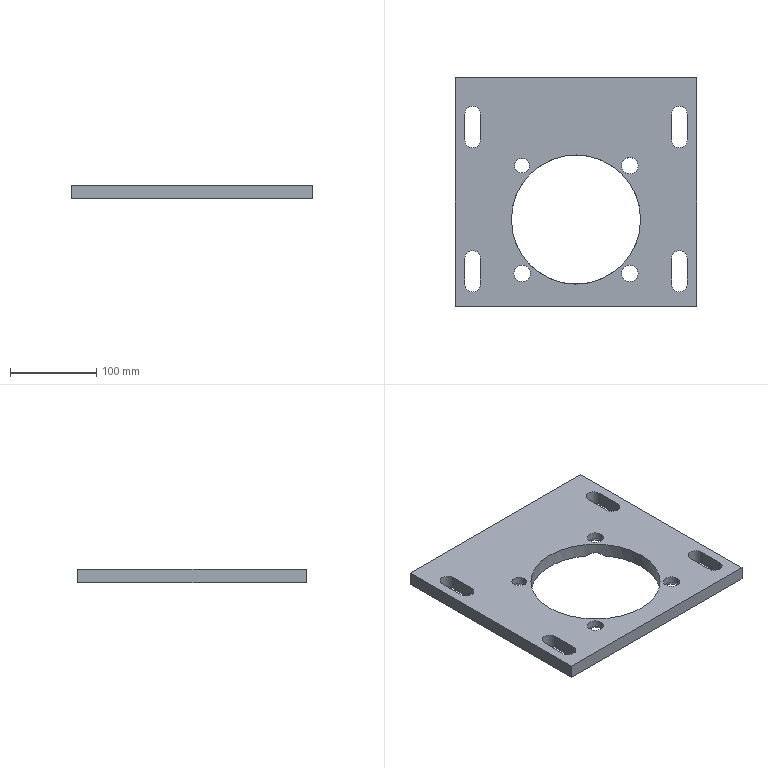Part | SolidWorks | features ICE 3, Extrusion 1 | 1 solid | 40 faces | box 280 x 265 x 16 mm | volume 827088 mm3 | cylinder 18 | plane 14 | cone 8 | commonest cylinder face diameters 18 x8 19 x6 17 x2 150 x2
STEP:
#1=CARTESIAN_POINT('',(-53.079,-62.579,0.));
#2=VERTEX_POINT('',#1);
#3=CARTESIAN_POINT('',(-72.079,-62.579,0.));
#4=VERTEX_POINT('',#3);
#5=CARTESIAN_POINT('',(-62.579,-62.579,0.));
#6=DIRECTION('',(0.,0.,1.));
#7=DIRECTION('',(1.,0.,0.));
#8=AXIS2_PLACEMENT_3D('',#5,#6,#7);
#9=CIRCLE('',#8,9.5);
#10=EDGE_CURVE('',#2,#4,#9,.T.);
#11=ORIENTED_EDGE('',*,*,#10,.T.);
#12=CARTESIAN_POINT('',(-80.079,-62.579,-8.));
#13=VERTEX_POINT('',#12);
#14=CARTESIAN_POINT('',(-72.079,-62.579,0.));
#15=DIRECTION('',(-0.7071,0.,-0.7071));
#16=VECTOR('',#15,1000.);
#17=LINE('',#14,#16);
#18=EDGE_CURVE('',#4,#13,#17,.T.);
#19=ORIENTED_EDGE('',*,*,#18,.T.);
#20=CARTESIAN_POINT('',(-59.769,-45.306,-8.));
#21=VERTEX_POINT('',#20);
#22=CARTESIAN_POINT('',(-62.579,-62.579,-8.));
#23=DIRECTION('',(0.,0.,1.));
#24=DIRECTION('',(1.,0.,0.));
#25=AXIS2_PLACEMENT_3D('',#22,#23,#24);
#26=CIRCLE('',#25,17.5);
#27=EDGE_CURVE('',#21,#13,#26,.T.);
#28=ORIENTED_EDGE('',*,*,#27,.F.);
#29=CARTESIAN_POINT('',(-45.306,-59.769,-8.));
#30=VERTEX_POINT('',#29);
#31=CARTESIAN_POINT('',(-59.769,-45.306,-8.));
#32=CARTESIAN_POINT('',(-59.304,-45.92,-7.469));
#33=CARTESIAN_POINT('',(-58.822,-46.537,-6.963));
#34=CARTESIAN_POINT('',(-57.811,-47.787,-6.028));
#35=CARTESIAN_POINT('',(-57.282,-48.42,-5.598));
#36=CARTESIAN_POINT('',(-56.442,-49.391,-5.041));
#37=CARTESIAN_POINT('',(-56.153,-49.72,-4.869));
#38=CARTESIAN_POINT('',(-55.56,-50.381,-4.567));
#39=CARTESIAN_POINT('',(-55.258,-50.712,-4.436));
#40=CARTESIAN_POINT('',(-54.642,-51.376,-4.223));
#41=CARTESIAN_POINT('',(-54.327,-51.708,-4.14));
#42=CARTESIAN_POINT('',(-53.685,-52.375,-4.028));
#43=CARTESIAN_POINT('',(-53.355,-52.711,-3.999));
#44=CARTESIAN_POINT('',(-52.358,-53.707,-4.001));
#45=CARTESIAN_POINT('',(-51.694,-54.346,-4.119));
#46=CARTESIAN_POINT('',(-50.697,-55.272,-4.442));
#47=CARTESIAN_POINT('',(-50.363,-55.576,-4.574));
#48=CARTESIAN_POINT('',(-49.702,-56.168,-4.878));
#49=CARTESIAN_POINT('',(-49.377,-56.455,-5.049));
#50=CARTESIAN_POINT('',(-48.41,-57.29,-5.604));
#51=CARTESIAN_POINT('',(-47.78,-57.816,-6.033));
#52=CARTESIAN_POINT('',(-46.534,-58.824,-6.966));
#53=CARTESIAN_POINT('',(-45.918,-59.305,-7.47));
#54=CARTESIAN_POINT('',(-45.306,-59.769,-8.));
#55=B_SPLINE_CURVE_WITH_KNOTS('',3,(#31,#32,#33,#34,#35,#36,#37,#38,#39,#40,#41,#42,#43,#44,#45,#46,#47,#48,#49,#50,#51,#52,#53,#54),.UNSPECIFIED.,.F.,.F.,(4,2,2,2,2,2,2,2,2,2,2,4),(0.00000035,0.002789,0.005578,0.006972,0.008366,0.009761,0.01116,0.01394,0.01534,0.01673,0.01952,0.02231),.UNSPECIFIED.);
#56=EDGE_CURVE('',#21,#30,#55,.T.);
#57=ORIENTED_EDGE('',*,*,#56,.T.);
#58=CARTESIAN_POINT('',(-45.079,-62.579,-8.));
#59=VERTEX_POINT('',#58);
#60=CARTESIAN_POINT('',(-62.579,-62.579,-8.));
#61=DIRECTION('',(0.,0.,1.));
#62=DIRECTION('',(1.,0.,0.));
#63=AXIS2_PLACEMENT_3D('',#60,#61,#62);
#64=CIRCLE('',#63,17.5);
#65=EDGE_CURVE('',#59,#30,#64,.T.);
#66=ORIENTED_EDGE('',*,*,#65,.F.);
#67=CARTESIAN_POINT('',(-53.079,-62.579,0.));
#68=DIRECTION('',(0.7071,0.,-0.7071));
#69=VECTOR('',#68,1000.);
#70=LINE('',#67,#69);
#71=EDGE_CURVE('',#2,#59,#70,.T.);
#72=ORIENTED_EDGE('',*,*,#71,.F.);
#73=EDGE_LOOP('',(#11,#19,#28,#57,#66,#72));
#74=FACE_OUTER_BOUND('',#73,.T.);
#75=CARTESIAN_POINT('',(-62.579,-62.579,0.));
#76=DIRECTION('',(0.,0.,-1.));
#77=DIRECTION('',(1.,0.,0.));
#78=AXIS2_PLACEMENT_3D('',#75,#76,#77);
#79=CONICAL_SURFACE('',#78,9.5,0.7854);
#80=ADVANCED_FACE('',(#74),#79,.F.);
#81=CARTESIAN_POINT('',(72.079,-62.579,0.));
#82=VERTEX_POINT('',#81);
#83=CARTESIAN_POINT('',(53.079,-62.579,0.));
#84=VERTEX_POINT('',#83);
#85=CARTESIAN_POINT('',(62.579,-62.579,0.));
#86=DIRECTION('',(0.,0.,1.));
#87=DIRECTION('',(1.,0.,0.));
#88=AXIS2_PLACEMENT_3D('',#85,#86,#87);
#89=CIRCLE('',#88,9.5);
#90=EDGE_CURVE('',#82,#84,#89,.T.);
#91=ORIENTED_EDGE('',*,*,#90,.T.);
#92=CARTESIAN_POINT('',(45.079,-62.579,-8.));
#93=VERTEX_POINT('',#92);
#94=CARTESIAN_POINT('',(53.079,-62.579,0.));
#95=DIRECTION('',(-0.7071,0.,-0.7071));
#96=VECTOR('',#95,1000.);
#97=LINE('',#94,#96);
#98=EDGE_CURVE('',#84,#93,#97,.T.);
#99=ORIENTED_EDGE('',*,*,#98,.T.);
#100=CARTESIAN_POINT('',(45.306,-59.769,-8.));
#101=VERTEX_POINT('',#100);
#102=CARTESIAN_POINT('',(62.579,-62.579,-8.));
#103=DIRECTION('',(0.,0.,1.));
#104=DIRECTION('',(1.,0.,0.));
#105=AXIS2_PLACEMENT_3D('',#102,#103,#104);
#106=CIRCLE('',#105,17.5);
#107=EDGE_CURVE('',#101,#93,#106,.T.);
#108=ORIENTED_EDGE('',*,*,#107,.F.);
#109=CARTESIAN_POINT('',(59.769,-45.306,-8.));
#110=VERTEX_POINT('',#109);
#111=CARTESIAN_POINT('',(45.306,-59.769,-8.));
#112=CARTESIAN_POINT('',(45.92,-59.304,-7.469));
#113=CARTESIAN_POINT('',(46.537,-58.822,-6.963));
#114=CARTESIAN_POINT('',(47.787,-57.811,-6.028));
#115=CARTESIAN_POINT('',(48.42,-57.282,-5.598));
#116=CARTESIAN_POINT('',(49.391,-56.442,-5.041));
#117=CARTESIAN_POINT('',(49.72,-56.153,-4.869));
#118=CARTESIAN_POINT('',(50.381,-55.56,-4.567));
#119=CARTESIAN_POINT('',(50.712,-55.258,-4.436));
#120=CARTESIAN_POINT('',(51.376,-54.642,-4.223));
#121=CARTESIAN_POINT('',(51.708,-54.327,-4.14));
#122=CARTESIAN_POINT('',(52.375,-53.685,-4.028));
#123=CARTESIAN_POINT('',(52.711,-53.355,-3.999));
#124=CARTESIAN_POINT('',(53.707,-52.358,-4.001));
#125=CARTESIAN_POINT('',(54.346,-51.694,-4.119));
#126=CARTESIAN_POINT('',(55.272,-50.697,-4.442));
#127=CARTESIAN_POINT('',(55.576,-50.363,-4.574));
#128=CARTESIAN_POINT('',(56.168,-49.702,-4.878));
#129=CARTESIAN_POINT('',(56.455,-49.377,-5.049));
#130=CARTESIAN_POINT('',(57.29,-48.41,-5.604));
#131=CARTESIAN_POINT('',(57.816,-47.78,-6.033));
#132=CARTESIAN_POINT('',(58.824,-46.534,-6.966));
#133=CARTESIAN_POINT('',(59.305,-45.918,-7.47));
#134=CARTESIAN_POINT('',(59.769,-45.306,-8.));
#135=B_SPLINE_CURVE_WITH_KNOTS('',3,(#111,#112,#113,#114,#115,#116,#117,#118,#119,#120,#121,#122,#123,#124,#125,#126,#127,#128,#129,#130,#131,#132,#133,#134),.UNSPECIFIED.,.F.,.F.,(4,2,2,2,2,2,2,2,2,2,2,4),(0.00000035,0.002789,0.005578,0.006972,0.008366,0.009761,0.01116,0.01394,0.01534,0.01673,0.01952,0.02231),.UNSPECIFIED.);
#136=EDGE_CURVE('',#101,#110,#135,.T.);
#137=ORIENTED_EDGE('',*,*,#136,.T.);
#138=CARTESIAN_POINT('',(80.079,-62.579,-8.));
#139=VERTEX_POINT('',#138);
#140=CARTESIAN_POINT('',(62.579,-62.579,-8.));
#141=DIRECTION('',(0.,0.,1.));
#142=DIRECTION('',(1.,0.,0.));
#143=AXIS2_PLACEMENT_3D('',#140,#141,#142);
#144=CIRCLE('',#143,17.5);
#145=EDGE_CURVE('',#139,#110,#144,.T.);
#146=ORIENTED_EDGE('',*,*,#145,.F.);
#147=CARTESIAN_POINT('',(72.079,-62.579,0.));
#148=DIRECTION('',(0.7071,0.,-0.7071));
#149=VECTOR('',#148,1000.);
#150=LINE('',#147,#149);
#151=EDGE_CURVE('',#82,#139,#150,.T.);
#152=ORIENTED_EDGE('',*,*,#151,.F.);
#153=EDGE_LOOP('',(#91,#99,#108,#137,#146,#152));
#154=FACE_OUTER_BOUND('',#153,.T.);
#155=CARTESIAN_POINT('',(62.579,-62.579,0.));
#156=DIRECTION('',(0.,0.,-1.));
#157=DIRECTION('',(1.,0.,0.));
#158=AXIS2_PLACEMENT_3D('',#155,#156,#157);
#159=CONICAL_SURFACE('',#158,9.5,0.7854);
#160=ADVANCED_FACE('',(#154),#159,.F.);
#161=CARTESIAN_POINT('',(72.079,62.579,0.));
#162=VERTEX_POINT('',#161);
#163=CARTESIAN_POINT('',(53.079,62.579,0.));
#164=VERTEX_POINT('',#163);
#165=CARTESIAN_POINT('',(62.579,62.579,0.));
#166=DIRECTION('',(0.,0.,1.));
#167=DIRECTION('',(1.,0.,0.));
#168=AXIS2_PLACEMENT_3D('',#165,#166,#167);
#169=CIRCLE('',#168,9.5);
#170=EDGE_CURVE('',#162,#164,#169,.T.);
#171=ORIENTED_EDGE('',*,*,#170,.T.);
#172=CARTESIAN_POINT('',(45.079,62.579,-8.));
#173=VERTEX_POINT('',#172);
#174=CARTESIAN_POINT('',(53.079,62.579,0.));
#175=DIRECTION('',(-0.7071,0.,-0.7071));
#176=VECTOR('',#175,1000.);
#177=LINE('',#174,#176);
#178=EDGE_CURVE('',#164,#173,#177,.T.);
#179=ORIENTED_EDGE('',*,*,#178,.T.);
#180=CARTESIAN_POINT('',(80.079,62.579,-8.));
#181=VERTEX_POINT('',#180);
#182=CARTESIAN_POINT('',(62.579,62.579,-8.));
#183=DIRECTION('',(0.,0.,1.));
#184=DIRECTION('',(1.,0.,0.));
#185=AXIS2_PLACEMENT_3D('',#182,#183,#184);
#186=CIRCLE('',#185,17.5);
#187=EDGE_CURVE('',#181,#173,#186,.T.);
#188=ORIENTED_EDGE('',*,*,#187,.F.);
#189=CARTESIAN_POINT('',(72.079,62.579,0.));
#190=DIRECTION('',(0.7071,0.,-0.7071));
#191=VECTOR('',#190,1000.);
#192=LINE('',#189,#191);
#193=EDGE_CURVE('',#162,#181,#192,.T.);
#194=ORIENTED_EDGE('',*,*,#193,.F.);
#195=EDGE_LOOP('',(#171,#179,#188,#194));
#196=FACE_OUTER_BOUND('',#195,.T.);
#197=CARTESIAN_POINT('',(62.579,62.579,0.));
#198=DIRECTION('',(0.,0.,-1.));
#199=DIRECTION('',(1.,0.,0.));
#200=AXIS2_PLACEMENT_3D('',#197,#198,#199);
#201=CONICAL_SURFACE('',#200,9.5,0.7854);
#202=ADVANCED_FACE('',(#196),#201,.F.);
#203=CARTESIAN_POINT('',(-54.079,62.579,0.));
#204=VERTEX_POINT('',#203);
#205=CARTESIAN_POINT('',(-71.079,62.579,0.));
#206=VERTEX_POINT('',#205);
#207=CARTESIAN_POINT('',(-62.579,62.579,0.));
#208=DIRECTION('',(0.,0.,1.));
#209=DIRECTION('',(1.,0.,0.));
#210=AXIS2_PLACEMENT_3D('',#207,#208,#209);
#211=CIRCLE('',#210,8.5);
#212=EDGE_CURVE('',#204,#206,#211,.T.);
#213=ORIENTED_EDGE('',*,*,#212,.T.);
#214=CARTESIAN_POINT('',(-79.079,62.579,-8.));
#215=VERTEX_POINT('',#214);
#216=CARTESIAN_POINT('',(-71.079,62.579,0.));
#217=DIRECTION('',(-0.7071,0.,-0.7071));
#218=VECTOR('',#217,1000.);
#219=LINE('',#216,#218);
#220=EDGE_CURVE('',#206,#215,#219,.T.);
#221=ORIENTED_EDGE('',*,*,#220,.T.);
#222=CARTESIAN_POINT('',(-46.079,62.579,-8.));
#223=VERTEX_POINT('',#222);
#224=CARTESIAN_POINT('',(-62.579,62.579,-8.));
#225=DIRECTION('',(0.,0.,1.));
#226=DIRECTION('',(1.,0.,0.));
#227=AXIS2_PLACEMENT_3D('',#224,#225,#226);
#228=CIRCLE('',#227,16.5);
#229=EDGE_CURVE('',#223,#215,#228,.T.);
#230=ORIENTED_EDGE('',*,*,#229,.F.);
#231=CARTESIAN_POINT('',(-54.079,62.579,0.));
#232=DIRECTION('',(0.7071,0.,-0.7071));
#233=VECTOR('',#232,1000.);
#234=LINE('',#231,#233);
#235=EDGE_CURVE('',#204,#223,#234,.T.);
#236=ORIENTED_EDGE('',*,*,#235,.F.);
#237=EDGE_LOOP('',(#213,#221,#230,#236));
#238=FACE_OUTER_BOUND('',#237,.T.);
#239=CARTESIAN_POINT('',(-62.579,62.579,0.));
#240=DIRECTION('',(0.,0.,-1.));
#241=DIRECTION('',(1.,0.,0.));
#242=AXIS2_PLACEMENT_3D('',#239,#240,#241);
#243=CONICAL_SURFACE('',#242,8.5,0.7854);
#244=ADVANCED_FACE('',(#238),#243,.F.);
#245=CARTESIAN_POINT('',(-62.579,-62.579,0.));
#246=DIRECTION('',(0.,0.,1.));
#247=DIRECTION('',(1.,0.,0.));
#248=AXIS2_PLACEMENT_3D('',#245,#246,#247);
#249=CIRCLE('',#248,9.5);
#250=EDGE_CURVE('',#4,#2,#249,.T.);
#251=ORIENTED_EDGE('',*,*,#250,.F.);
#252=CARTESIAN_POINT('',(-72.079,-62.579,8.));
#253=VERTEX_POINT('',#252);
#254=CARTESIAN_POINT('',(-72.079,-62.579,0.));
#255=DIRECTION('',(0.,0.,1.));
#256=VECTOR('',#255,1000.);
#257=LINE('',#254,#256);
#258=EDGE_CURVE('',#4,#253,#257,.T.);
#259=ORIENTED_EDGE('',*,*,#258,.T.);
#260=CARTESIAN_POINT('',(-53.079,-62.579,8.));
#261=VERTEX_POINT('',#260);
#262=CARTESIAN_POINT('',(-62.579,-62.579,8.));
#263=DIRECTION('',(0.,0.,1.));
#264=DIRECTION('',(1.,0.,0.));
#265=AXIS2_PLACEMENT_3D('',#262,#263,#264);
#266=CIRCLE('',#265,9.5);
#267=EDGE_CURVE('',#253,#261,#266,.T.);
#268=ORIENTED_EDGE('',*,*,#267,.T.);
#269=CARTESIAN_POINT('',(-53.079,-62.579,0.));
#270=DIRECTION('',(0.,0.,1.));
#271=VECTOR('',#270,1000.);
#272=LINE('',#269,#271);
#273=EDGE_CURVE('',#2,#261,#272,.T.);
#274=ORIENTED_EDGE('',*,*,#273,.F.);
#275=EDGE_LOOP('',(#251,#259,#268,#274));
#276=FACE_OUTER_BOUND('',#275,.T.);
#277=CARTESIAN_POINT('',(-62.579,-62.579,0.));
#278=DIRECTION('',(0.,0.,1.));
#279=DIRECTION('',(1.,0.,0.));
#280=AXIS2_PLACEMENT_3D('',#277,#278,#279);
#281=CYLINDRICAL_SURFACE('',#280,9.5);
#282=ADVANCED_FACE('',(#276),#281,.F.);
#283=CARTESIAN_POINT('',(62.579,-62.579,0.));
#284=DIRECTION('',(0.,0.,1.));
#285=DIRECTION('',(1.,0.,0.));
#286=AXIS2_PLACEMENT_3D('',#283,#284,#285);
#287=CIRCLE('',#286,9.5);
#288=EDGE_CURVE('',#84,#82,#287,.T.);
#289=ORIENTED_EDGE('',*,*,#288,.F.);
#290=CARTESIAN_POINT('',(53.079,-62.579,8.));
#291=VERTEX_POINT('',#290);
#292=CARTESIAN_POINT('',(53.079,-62.579,0.));
#293=DIRECTION('',(0.,0.,1.));
#294=VECTOR('',#293,1000.);
#295=LINE('',#292,#294);
#296=EDGE_CURVE('',#84,#291,#295,.T.);
#297=ORIENTED_EDGE('',*,*,#296,.T.);
#298=CARTESIAN_POINT('',(72.079,-62.579,8.));
#299=VERTEX_POINT('',#298);
#300=CARTESIAN_POINT('',(62.579,-62.579,8.));
#301=DIRECTION('',(0.,0.,1.));
#302=DIRECTION('',(1.,0.,0.));
#303=AXIS2_PLACEMENT_3D('',#300,#301,#302);
#304=CIRCLE('',#303,9.5);
#305=EDGE_CURVE('',#291,#299,#304,.T.);
#306=ORIENTED_EDGE('',*,*,#305,.T.);
#307=CARTESIAN_POINT('',(72.079,-62.579,0.));
#308=DIRECTION('',(0.,0.,1.));
#309=VECTOR('',#308,1000.);
#310=LINE('',#307,#309);
#311=EDGE_CURVE('',#82,#299,#310,.T.);
#312=ORIENTED_EDGE('',*,*,#311,.F.);
#313=EDGE_LOOP('',(#289,#297,#306,#312));
#314=FACE_OUTER_BOUND('',#313,.T.);
#315=CARTESIAN_POINT('',(62.579,-62.579,0.));
#316=DIRECTION('',(0.,0.,1.));
#317=DIRECTION('',(1.,0.,0.));
#318=AXIS2_PLACEMENT_3D('',#315,#316,#317);
#319=CYLINDRICAL_SURFACE('',#318,9.5);
#320=ADVANCED_FACE('',(#314),#319,.F.);
#321=CARTESIAN_POINT('',(62.579,62.579,0.));
#322=DIRECTION('',(0.,0.,1.));
#323=DIRECTION('',(1.,0.,0.));
#324=AXIS2_PLACEMENT_3D('',#321,#322,#323);
#325=CIRCLE('',#324,9.5);
#326=EDGE_CURVE('',#164,#162,#325,.T.);
#327=ORIENTED_EDGE('',*,*,#326,.F.);
#328=CARTESIAN_POINT('',(53.079,62.579,8.));
#329=VERTEX_POINT('',#328);
#330=CARTESIAN_POINT('',(53.079,62.579,0.));
#331=DIRECTION('',(0.,0.,1.));
#332=VECTOR('',#331,1000.);
#333=LINE('',#330,#332);
#334=EDGE_CURVE('',#164,#329,#333,.T.);
#335=ORIENTED_EDGE('',*,*,#334,.T.);
#336=CARTESIAN_POINT('',(72.079,62.579,8.));
#337=VERTEX_POINT('',#336);
#338=CARTESIAN_POINT('',(62.579,62.579,8.));
#339=DIRECTION('',(0.,0.,1.));
#340=DIRECTION('',(1.,0.,0.));
#341=AXIS2_PLACEMENT_3D('',#338,#339,#340);
#342=CIRCLE('',#341,9.5);
#343=EDGE_CURVE('',#329,#337,#342,.T.);
#344=ORIENTED_EDGE('',*,*,#343,.T.);
#345=CARTESIAN_POINT('',(72.079,62.579,0.));
#346=DIRECTION('',(0.,0.,1.));
#347=VECTOR('',#346,1000.);
#348=LINE('',#345,#347);
#349=EDGE_CURVE('',#162,#337,#348,.T.);
#350=ORIENTED_EDGE('',*,*,#349,.F.);
#351=EDGE_LOOP('',(#327,#335,#344,#350));
#352=FACE_OUTER_BOUND('',#351,.T.);
#353=CARTESIAN_POINT('',(62.579,62.579,0.));
#354=DIRECTION('',(0.,0.,1.));
#355=DIRECTION('',(1.,0.,0.));
#356=AXIS2_PLACEMENT_3D('',#353,#354,#355);
#357=CYLINDRICAL_SURFACE('',#356,9.5);
#358=ADVANCED_FACE('',(#352),#357,.F.);
#359=CARTESIAN_POINT('',(-62.579,62.579,0.));
#360=DIRECTION('',(0.,0.,1.));
#361=DIRECTION('',(1.,0.,0.));
#362=AXIS2_PLACEMENT_3D('',#359,#360,#361);
#363=CIRCLE('',#362,8.5);
#364=EDGE_CURVE('',#206,#204,#363,.T.);
#365=ORIENTED_EDGE('',*,*,#364,.F.);
#366=CARTESIAN_POINT('',(-71.079,62.579,8.));
#367=VERTEX_POINT('',#366);
#368=CARTESIAN_POINT('',(-71.079,62.579,0.));
#369=DIRECTION('',(0.,0.,1.));
#370=VECTOR('',#369,1000.);
#371=LINE('',#368,#370);
#372=EDGE_CURVE('',#206,#367,#371,.T.);
#373=ORIENTED_EDGE('',*,*,#372,.T.);
#374=CARTESIAN_POINT('',(-54.079,62.579,8.));
#375=VERTEX_POINT('',#374);
#376=CARTESIAN_POINT('',(-62.579,62.579,8.));
#377=DIRECTION('',(0.,0.,1.));
#378=DIRECTION('',(1.,0.,0.));
#379=AXIS2_PLACEMENT_3D('',#376,#377,#378);
#380=CIRCLE('',#379,8.5);
#381=EDGE_CURVE('',#367,#375,#380,.T.);
#382=ORIENTED_EDGE('',*,*,#381,.T.);
#383=CARTESIAN_POINT('',(-54.079,62.579,0.));
#384=DIRECTION('',(0.,0.,1.));
#385=VECTOR('',#384,1000.);
#386=LINE('',#383,#385);
#387=EDGE_CURVE('',#204,#375,#386,.T.);
#388=ORIENTED_EDGE('',*,*,#387,.F.);
#389=EDGE_LOOP('',(#365,#373,#382,#388));
#390=FACE_OUTER_BOUND('',#389,.T.);
#391=CARTESIAN_POINT('',(-62.579,62.579,0.));
#392=DIRECTION('',(0.,0.,1.));
#393=DIRECTION('',(1.,0.,0.));
#394=AXIS2_PLACEMENT_3D('',#391,#392,#393);
#395=CYLINDRICAL_SURFACE('',#394,8.5);
#396=ADVANCED_FACE('',(#390),#395,.F.);
#397=CARTESIAN_POINT('',(-75.,0.,8.));
#398=VERTEX_POINT('',#397);
#399=CARTESIAN_POINT('',(75.,0.,8.));
#400=VERTEX_POINT('',#399);
#401=CARTESIAN_POINT('',(0.,0.,8.));
#402=DIRECTION('',(0.,0.,1.));
#403=DIRECTION('',(1.,0.,0.));
#404=AXIS2_PLACEMENT_3D('',#401,#402,#403);
#405=CIRCLE('',#404,75.);
#406=EDGE_CURVE('',#398,#400,#405,.T.);
#407=ORIENTED_EDGE('',*,*,#406,.T.);
#408=CARTESIAN_POINT('',(75.,0.,-8.));
#409=VERTEX_POINT('',#408);
#410=CARTESIAN_POINT('',(75.,0.,8.));
#411=DIRECTION('',(0.,0.,-1.));
#412=VECTOR('',#411,1000.);
#413=LINE('',#410,#412);
#414=EDGE_CURVE('',#400,#409,#413,.T.);
#415=ORIENTED_EDGE('',*,*,#414,.T.);
#416=CARTESIAN_POINT('',(0.,0.,-8.));
#417=DIRECTION('',(0.,0.,1.));
#418=DIRECTION('',(1.,0.,0.));
#419=AXIS2_PLACEMENT_3D('',#416,#417,#418);
#420=CIRCLE('',#419,75.);
#421=EDGE_CURVE('',#110,#409,#420,.T.);
#422=ORIENTED_EDGE('',*,*,#421,.F.);
#423=ORIENTED_EDGE('',*,*,#136,.F.);
#424=CARTESIAN_POINT('',(0.,0.,-8.));
#425=DIRECTION('',(0.,0.,1.));
#426=DIRECTION('',(1.,0.,0.));
#427=AXIS2_PLACEMENT_3D('',#424,#425,#426);
#428=CIRCLE('',#427,75.);
#429=EDGE_CURVE('',#30,#101,#428,.T.);
#430=ORIENTED_EDGE('',*,*,#429,.F.);
#431=ORIENTED_EDGE('',*,*,#56,.F.);
#432=CARTESIAN_POINT('',(-75.,0.,-8.));
#433=VERTEX_POINT('',#432);
#434=CARTESIAN_POINT('',(0.,0.,-8.));
#435=DIRECTION('',(0.,0.,1.));
#436=DIRECTION('',(1.,0.,0.));
#437=AXIS2_PLACEMENT_3D('',#434,#435,#436);
#438=CIRCLE('',#437,75.);
#439=EDGE_CURVE('',#433,#21,#438,.T.);
#440=ORIENTED_EDGE('',*,*,#439,.F.);
#441=CARTESIAN_POINT('',(-75.,0.,8.));
#442=DIRECTION('',(0.,0.,-1.));
#443=VECTOR('',#442,1000.);
#444=LINE('',#441,#443);
#445=EDGE_CURVE('',#398,#433,#444,.T.);
#446=ORIENTED_EDGE('',*,*,#445,.F.);
#447=EDGE_LOOP('',(#407,#415,#422,#423,#430,#431,#440,#446));
#448=FACE_OUTER_BOUND('',#447,.T.);
#449=CARTESIAN_POINT('',(0.,0.,8.));
#450=DIRECTION('',(0.,0.,-1.));
#451=DIRECTION('',(-1.,0.,0.));
#452=AXIS2_PLACEMENT_3D('',#449,#450,#451);
#453=CYLINDRICAL_SURFACE('',#452,75.);
#454=ADVANCED_FACE('',(#448),#453,.F.);
#455=CARTESIAN_POINT('',(140.,-100.5,8.));
#456=VERTEX_POINT('',#455);
#457=CARTESIAN_POINT('',(-140.,-100.5,8.));
#458=VERTEX_POINT('',#457);
#459=CARTESIAN_POINT('',(-140.,-100.5,8.));
#460=DIRECTION('',(-1.,0.,0.));
#461=VECTOR('',#460,1000.);
#462=LINE('',#459,#461);
#463=EDGE_CURVE('',#456,#458,#462,.T.);
#464=ORIENTED_EDGE('',*,*,#463,.F.);
#465=CARTESIAN_POINT('',(140.,164.5,8.));
#466=VERTEX_POINT('',#465);
#467=CARTESIAN_POINT('',(140.,-115.5,8.));
#468=DIRECTION('',(0.,1.,0.));
#469=VECTOR('',#468,1000.);
#470=LINE('',#467,#469);
#471=EDGE_CURVE('',#456,#466,#470,.T.);
#472=ORIENTED_EDGE('',*,*,#471,.T.);
#473=CARTESIAN_POINT('',(-140.,164.5,8.));
#474=VERTEX_POINT('',#473);
#475=CARTESIAN_POINT('',(140.,164.5,8.));
#476=DIRECTION('',(-1.,0.,0.));
#477=VECTOR('',#476,1000.);
#478=LINE('',#475,#477);
#479=EDGE_CURVE('',#466,#474,#478,.T.);
#480=ORIENTED_EDGE('',*,*,#479,.T.);
#481=CARTESIAN_POINT('',(-140.,164.5,8.));
#482=DIRECTION('',(0.,-1.,0.));
#483=VECTOR('',#482,1000.);
#484=LINE('',#481,#483);
#485=EDGE_CURVE('',#474,#458,#484,.T.);
#486=ORIENTED_EDGE('',*,*,#485,.T.);
#487=EDGE_LOOP('',(#464,#472,#480,#486));
#488=FACE_OUTER_BOUND('',#487,.T.);
#489=CARTESIAN_POINT('',(-62.579,-62.579,8.));
#490=DIRECTION('',(0.,0.,1.));
#491=DIRECTION('',(1.,0.,0.));
#492=AXIS2_PLACEMENT_3D('',#489,#490,#491);
#493=CIRCLE('',#492,9.5);
#494=EDGE_CURVE('',#261,#253,#493,.T.);
#495=ORIENTED_EDGE('',*,*,#494,.F.);
#496=ORIENTED_EDGE('',*,*,#267,.F.);
#497=EDGE_LOOP('',(#495,#496));
#498=FACE_BOUND('',#497,.T.);
#499=CARTESIAN_POINT('',(62.579,-62.579,8.));
#500=DIRECTION('',(0.,0.,1.));
#501=DIRECTION('',(1.,0.,0.));
#502=AXIS2_PLACEMENT_3D('',#499,#500,#501);
#503=CIRCLE('',#502,9.5);
#504=EDGE_CURVE('',#299,#291,#503,.T.);
#505=ORIENTED_EDGE('',*,*,#504,.F.);
#506=ORIENTED_EDGE('',*,*,#305,.F.);
#507=EDGE_LOOP('',(#505,#506));
#508=FACE_BOUND('',#507,.T.);
#509=CARTESIAN_POINT('',(62.579,62.579,8.));
#510=DIRECTION('',(0.,0.,1.));
#511=DIRECTION('',(1.,0.,0.));
#512=AXIS2_PLACEMENT_3D('',#509,#510,#511);
#513=CIRCLE('',#512,9.5);
#514=EDGE_CURVE('',#337,#329,#513,.T.);
#515=ORIENTED_EDGE('',*,*,#514,.F.);
#516=ORIENTED_EDGE('',*,*,#343,.F.);
#517=EDGE_LOOP('',(#515,#516));
#518=FACE_BOUND('',#517,.T.);
#519=CARTESIAN_POINT('',(-62.579,62.579,8.));
#520=DIRECTION('',(0.,0.,1.));
#521=DIRECTION('',(1.,0.,0.));
#522=AXIS2_PLACEMENT_3D('',#519,#520,#521);
#523=CIRCLE('',#522,8.5);
#524=EDGE_CURVE('',#375,#367,#523,.T.);
#525=ORIENTED_EDGE('',*,*,#524,.F.);
#526=ORIENTED_EDGE('',*,*,#381,.F.);
#527=EDGE_LOOP('',(#525,#526));
#528=FACE_BOUND('',#527,.T.);
#529=CARTESIAN_POINT('',(-111.,-75.,8.));
#530=VERTEX_POINT('',#529);
#531=CARTESIAN_POINT('',(-111.,-45.,8.));
#532=VERTEX_POINT('',#531);
#533=CARTESIAN_POINT('',(-111.,-45.,8.));
#534=DIRECTION('',(0.,1.,0.));
#535=VECTOR('',#534,1000.);
#536=LINE('',#533,#535);
#537=EDGE_CURVE('',#530,#532,#536,.T.);
#538=ORIENTED_EDGE('',*,*,#537,.F.);
#539=CARTESIAN_POINT('',(-129.,-75.,8.));
#540=VERTEX_POINT('',#539);
#541=CARTESIAN_POINT('',(-120.,-75.,8.));
#542=DIRECTION('',(0.,0.,1.));
#543=DIRECTION('',(1.,0.,0.));
#544=AXIS2_PLACEMENT_3D('',#541,#542,#543);
#545=CIRCLE('',#544,9.);
#546=EDGE_CURVE('',#540,#530,#545,.T.);
#547=ORIENTED_EDGE('',*,*,#546,.F.);
#548=CARTESIAN_POINT('',(-129.,-45.,8.));
#549=VERTEX_POINT('',#548);
#550=CARTESIAN_POINT('',(-129.,-45.,8.));
#551=DIRECTION('',(0.,-1.,0.));
#552=VECTOR('',#551,1000.);
#553=LINE('',#550,#552);
#554=EDGE_CURVE('',#549,#540,#553,.T.);
#555=ORIENTED_EDGE('',*,*,#554,.F.);
#556=CARTESIAN_POINT('',(-120.,-45.,8.));
#557=DIRECTION('',(0.,0.,1.));
#558=DIRECTION('',(-1.,0.,0.));
#559=AXIS2_PLACEMENT_3D('',#556,#557,#558);
#560=CIRCLE('',#559,9.);
#561=EDGE_CURVE('',#532,#549,#560,.T.);
#562=ORIENTED_EDGE('',*,*,#561,.F.);
#563=EDGE_LOOP('',(#538,#547,#555,#562));
#564=FACE_BOUND('',#563,.T.);
#565=CARTESIAN_POINT('',(-111.,92.5,8.));
#566=VERTEX_POINT('',#565);
#567=CARTESIAN_POINT('',(-111.,122.5,8.));
#568=VERTEX_POINT('',#567);
#569=CARTESIAN_POINT('',(-111.,122.5,8.));
#570=DIRECTION('',(0.,1.,0.));
#571=VECTOR('',#570,1000.);
#572=LINE('',#569,#571);
#573=EDGE_CURVE('',#566,#568,#572,.T.);
#574=ORIENTED_EDGE('',*,*,#573,.F.);
#575=CARTESIAN_POINT('',(-129.,92.5,8.));
#576=VERTEX_POINT('',#575);
#577=CARTESIAN_POINT('',(-120.,92.5,8.));
#578=DIRECTION('',(0.,0.,1.));
#579=DIRECTION('',(1.,0.,0.));
#580=AXIS2_PLACEMENT_3D('',#577,#578,#579);
#581=CIRCLE('',#580,9.);
#582=EDGE_CURVE('',#576,#566,#581,.T.);
#583=ORIENTED_EDGE('',*,*,#582,.F.);
#584=CARTESIAN_POINT('',(-129.,122.5,8.));
#585=VERTEX_POINT('',#584);
#586=CARTESIAN_POINT('',(-129.,122.5,8.));
#587=DIRECTION('',(0.,-1.,0.));
#588=VECTOR('',#587,1000.);
#589=LINE('',#586,#588);
#590=EDGE_CURVE('',#585,#576,#589,.T.);
#591=ORIENTED_EDGE('',*,*,#590,.F.);
#592=CARTESIAN_POINT('',(-120.,122.5,8.));
#593=DIRECTION('',(0.,0.,1.));
#594=DIRECTION('',(-1.,0.,0.));
#595=AXIS2_PLACEMENT_3D('',#592,#593,#594);
#596=CIRCLE('',#595,9.);
#597=EDGE_CURVE('',#568,#585,#596,.T.);
#598=ORIENTED_EDGE('',*,*,#597,.F.);
#599=EDGE_LOOP('',(#574,#583,#591,#598));
#600=FACE_BOUND('',#599,.T.);
#601=ORIENTED_EDGE('',*,*,#406,.F.);
#602=CARTESIAN_POINT('',(0.,0.,8.));
#603=DIRECTION('',(0.,0.,1.));
#604=DIRECTION('',(1.,0.,0.));
#605=AXIS2_PLACEMENT_3D('',#602,#603,#604);
#606=CIRCLE('',#605,75.);
#607=EDGE_CURVE('',#400,#398,#606,.T.);
#608=ORIENTED_EDGE('',*,*,#607,.F.);
#609=EDGE_LOOP('',(#601,#608));
#610=FACE_BOUND('',#609,.T.);
#611=CARTESIAN_POINT('',(129.,92.5,8.));
#612=VERTEX_POINT('',#611);
#613=CARTESIAN_POINT('',(129.,122.5,8.));
#614=VERTEX_POINT('',#613);
#615=CARTESIAN_POINT('',(129.,122.5,8.));
#616=DIRECTION('',(0.,1.,0.));
#617=VECTOR('',#616,1000.);
#618=LINE('',#615,#617);
#619=EDGE_CURVE('',#612,#614,#618,.T.);
#620=ORIENTED_EDGE('',*,*,#619,.F.);
#621=CARTESIAN_POINT('',(111.,92.5,8.));
#622=VERTEX_POINT('',#621);
#623=CARTESIAN_POINT('',(120.,92.5,8.));
#624=DIRECTION('',(0.,0.,1.));
#625=DIRECTION('',(1.,0.,0.));
#626=AXIS2_PLACEMENT_3D('',#623,#624,#625);
#627=CIRCLE('',#626,9.);
#628=EDGE_CURVE('',#622,#612,#627,.T.);
#629=ORIENTED_EDGE('',*,*,#628,.F.);
#630=CARTESIAN_POINT('',(111.,122.5,8.));
#631=VERTEX_POINT('',#630);
#632=CARTESIAN_POINT('',(111.,122.5,8.));
#633=DIRECTION('',(0.,-1.,0.));
#634=VECTOR('',#633,1000.);
#635=LINE('',#632,#634);
#636=EDGE_CURVE('',#631,#622,#635,.T.);
#637=ORIENTED_EDGE('',*,*,#636,.F.);
#638=CARTESIAN_POINT('',(120.,122.5,8.));
#639=DIRECTION('',(0.,0.,1.));
#640=DIRECTION('',(-1.,0.,0.));
#641=AXIS2_PLACEMENT_3D('',#638,#639,#640);
#642=CIRCLE('',#641,9.);
#643=EDGE_CURVE('',#614,#631,#642,.T.);
#644=ORIENTED_EDGE('',*,*,#643,.F.);
#645=EDGE_LOOP('',(#620,#629,#637,#644));
#646=FACE_BOUND('',#645,.T.);
#647=CARTESIAN_POINT('',(129.,-75.,8.));
#648=VERTEX_POINT('',#647);
#649=CARTESIAN_POINT('',(129.,-45.,8.));
#650=VERTEX_POINT('',#649);
#651=CARTESIAN_POINT('',(129.,-45.,8.));
#652=DIRECTION('',(0.,1.,0.));
#653=VECTOR('',#652,1000.);
#654=LINE('',#651,#653);
#655=EDGE_CURVE('',#648,#650,#654,.T.);
#656=ORIENTED_EDGE('',*,*,#655,.F.);
#657=CARTESIAN_POINT('',(111.,-75.,8.));
#658=VERTEX_POINT('',#657);
#659=CARTESIAN_POINT('',(120.,-75.,8.));
#660=DIRECTION('',(0.,0.,1.));
#661=DIRECTION('',(1.,0.,0.));
#662=AXIS2_PLACEMENT_3D('',#659,#660,#661);
#663=CIRCLE('',#662,9.);
#664=EDGE_CURVE('',#658,#648,#663,.T.);
#665=ORIENTED_EDGE('',*,*,#664,.F.);
#666=CARTESIAN_POINT('',(111.,-45.,8.));
#667=VERTEX_POINT('',#666);
#668=CARTESIAN_POINT('',(111.,-45.,8.));
#669=DIRECTION('',(0.,-1.,0.));
#670=VECTOR('',#669,1000.);
#671=LINE('',#668,#670);
#672=EDGE_CURVE('',#667,#658,#671,.T.);
#673=ORIENTED_EDGE('',*,*,#672,.F.);
#674=CARTESIAN_POINT('',(120.,-45.,8.));
#675=DIRECTION('',(0.,0.,1.));
#676=DIRECTION('',(-1.,0.,0.));
#677=AXIS2_PLACEMENT_3D('',#674,#675,#676);
#678=CIRCLE('',#677,9.);
#679=EDGE_CURVE('',#650,#667,#678,.T.);
#680=ORIENTED_EDGE('',*,*,#679,.F.);
#681=EDGE_LOOP('',(#656,#665,#673,#680));
#682=FACE_BOUND('',#681,.T.);
#683=CARTESIAN_POINT('',(-140.,164.5,8.));
#684=DIRECTION('',(0.,0.,1.));
#685=DIRECTION('',(1.,0.,0.));
#686=AXIS2_PLACEMENT_3D('',#683,#684,#685);
#687=PLANE('',#686);
#688=ADVANCED_FACE('',(#488,#498,#508,#518,#528,#564,#600,#610,#646,#682),#687,.T.);
#689=CARTESIAN_POINT('',(-129.,-75.,-8.));
#690=VERTEX_POINT('',#689);
#691=CARTESIAN_POINT('',(-111.,-75.,-8.));
#692=VERTEX_POINT('',#691);
#693=CARTESIAN_POINT('',(-120.,-75.,-8.));
#694=DIRECTION('',(0.,0.,1.));
#695=DIRECTION('',(1.,0.,0.));
#696=AXIS2_PLACEMENT_3D('',#693,#694,#695);
#697=CIRCLE('',#696,9.);
#698=EDGE_CURVE('',#690,#692,#697,.T.);
#699=ORIENTED_EDGE('',*,*,#698,.T.);
#700=CARTESIAN_POINT('',(-111.,-45.,-8.));
#701=VERTEX_POINT('',#700);
#702=CARTESIAN_POINT('',(-111.,-45.,-8.));
#703=DIRECTION('',(0.,1.,0.));
#704=VECTOR('',#703,1000.);
#705=LINE('',#702,#704);
#706=EDGE_CURVE('',#692,#701,#705,.T.);
#707=ORIENTED_EDGE('',*,*,#706,.T.);
#708=CARTESIAN_POINT('',(-129.,-45.,-8.));
#709=VERTEX_POINT('',#708);
#710=CARTESIAN_POINT('',(-120.,-45.,-8.));
#711=DIRECTION('',(0.,0.,1.));
#712=DIRECTION('',(-1.,0.,0.));
#713=AXIS2_PLACEMENT_3D('',#710,#711,#712);
#714=CIRCLE('',#713,9.);
#715=EDGE_CURVE('',#701,#709,#714,.T.);
#716=ORIENTED_EDGE('',*,*,#715,.T.);
#717=CARTESIAN_POINT('',(-129.,-45.,-8.));
#718=DIRECTION('',(0.,-1.,0.));
#719=VECTOR('',#718,1000.);
#720=LINE('',#717,#719);
#721=EDGE_CURVE('',#709,#690,#720,.T.);
#722=ORIENTED_EDGE('',*,*,#721,.T.);
#723=EDGE_LOOP('',(#699,#707,#716,#722));
#724=FACE_BOUND('',#723,.T.);
#725=CARTESIAN_POINT('',(-129.,92.5,-8.));
#726=VERTEX_POINT('',#725);
#727=CARTESIAN_POINT('',(-111.,92.5,-8.));
#728=VERTEX_POINT('',#727);
#729=CARTESIAN_POINT('',(-120.,92.5,-8.));
#730=DIRECTION('',(0.,0.,1.));
#731=DIRECTION('',(1.,0.,0.));
#732=AXIS2_PLACEMENT_3D('',#729,#730,#731);
#733=CIRCLE('',#732,9.);
#734=EDGE_CURVE('',#726,#728,#733,.T.);
#735=ORIENTED_EDGE('',*,*,#734,.T.);
#736=CARTESIAN_POINT('',(-111.,122.5,-8.));
#737=VERTEX_POINT('',#736);
#738=CARTESIAN_POINT('',(-111.,122.5,-8.));
#739=DIRECTION('',(0.,1.,0.));
#740=VECTOR('',#739,1000.);
#741=LINE('',#738,#740);
#742=EDGE_CURVE('',#728,#737,#741,.T.);
#743=ORIENTED_EDGE('',*,*,#742,.T.);
#744=CARTESIAN_POINT('',(-129.,122.5,-8.));
#745=VERTEX_POINT('',#744);
#746=CARTESIAN_POINT('',(-120.,122.5,-8.));
#747=DIRECTION('',(0.,0.,1.));
#748=DIRECTION('',(-1.,0.,0.));
#749=AXIS2_PLACEMENT_3D('',#746,#747,#748);
#750=CIRCLE('',#749,9.);
#751=EDGE_CURVE('',#737,#745,#750,.T.);
#752=ORIENTED_EDGE('',*,*,#751,.T.);
#753=CARTESIAN_POINT('',(-129.,122.5,-8.));
#754=DIRECTION('',(0.,-1.,0.));
#755=VECTOR('',#754,1000.);
#756=LINE('',#753,#755);
#757=EDGE_CURVE('',#745,#726,#756,.T.);
#758=ORIENTED_EDGE('',*,*,#757,.T.);
#759=EDGE_LOOP('',(#735,#743,#752,#758));
#760=FACE_BOUND('',#759,.T.);
#761=CARTESIAN_POINT('',(140.,-100.5,-8.));
#762=VERTEX_POINT('',#761);
#763=CARTESIAN_POINT('',(140.,164.5,-8.));
#764=VERTEX_POINT('',#763);
#765=CARTESIAN_POINT('',(140.,-115.5,-8.));
#766=DIRECTION('',(0.,1.,0.));
#767=VECTOR('',#766,1000.);
#768=LINE('',#765,#767);
#769=EDGE_CURVE('',#762,#764,#768,.T.);
#770=ORIENTED_EDGE('',*,*,#769,.F.);
#771=CARTESIAN_POINT('',(-140.,-100.5,-8.));
#772=VERTEX_POINT('',#771);
#773=CARTESIAN_POINT('',(-140.,-100.5,-8.));
#774=DIRECTION('',(-1.,0.,0.));
#775=VECTOR('',#774,1000.);
#776=LINE('',#773,#775);
#777=EDGE_CURVE('',#762,#772,#776,.T.);
#778=ORIENTED_EDGE('',*,*,#777,.T.);
#779=CARTESIAN_POINT('',(-140.,164.5,-8.));
#780=VERTEX_POINT('',#779);
#781=CARTESIAN_POINT('',(-140.,164.5,-8.));
#782=DIRECTION('',(0.,-1.,0.));
#783=VECTOR('',#782,1000.);
#784=LINE('',#781,#783);
#785=EDGE_CURVE('',#780,#772,#784,.T.);
#786=ORIENTED_EDGE('',*,*,#785,.F.);
#787=CARTESIAN_POINT('',(140.,164.5,-8.));
#788=DIRECTION('',(-1.,0.,0.));
#789=VECTOR('',#788,1000.);
#790=LINE('',#787,#789);
#791=EDGE_CURVE('',#764,#780,#790,.T.);
#792=ORIENTED_EDGE('',*,*,#791,.F.);
#793=EDGE_LOOP('',(#770,#778,#786,#792));
#794=FACE_OUTER_BOUND('',#793,.T.);
#795=CARTESIAN_POINT('',(-58.838,46.509,-8.));
#796=VERTEX_POINT('',#795);
#797=CARTESIAN_POINT('',(0.,0.,-8.));
#798=DIRECTION('',(0.,0.,1.));
#799=DIRECTION('',(1.,0.,0.));
#800=AXIS2_PLACEMENT_3D('',#797,#798,#799);
#801=CIRCLE('',#800,75.);
#802=EDGE_CURVE('',#796,#433,#801,.T.);
#803=ORIENTED_EDGE('',*,*,#802,.T.);
#804=ORIENTED_EDGE('',*,*,#439,.T.);
#805=ORIENTED_EDGE('',*,*,#27,.T.);
#806=CARTESIAN_POINT('',(-62.579,-62.579,-8.));
#807=DIRECTION('',(0.,0.,1.));
#808=DIRECTION('',(1.,0.,0.));
#809=AXIS2_PLACEMENT_3D('',#806,#807,#808);
#810=CIRCLE('',#809,17.5);
#811=EDGE_CURVE('',#13,#59,#810,.T.);
#812=ORIENTED_EDGE('',*,*,#811,.T.);
#813=ORIENTED_EDGE('',*,*,#65,.T.);
#814=ORIENTED_EDGE('',*,*,#429,.T.);
#815=ORIENTED_EDGE('',*,*,#107,.T.);
#816=CARTESIAN_POINT('',(62.579,-62.579,-8.));
#817=DIRECTION('',(0.,0.,1.));
#818=DIRECTION('',(1.,0.,0.));
#819=AXIS2_PLACEMENT_3D('',#816,#817,#818);
#820=CIRCLE('',#819,17.5);
#821=EDGE_CURVE('',#93,#139,#820,.T.);
#822=ORIENTED_EDGE('',*,*,#821,.T.);
#823=ORIENTED_EDGE('',*,*,#145,.T.);
#824=ORIENTED_EDGE('',*,*,#421,.T.);
#825=CARTESIAN_POINT('',(59.769,45.306,-8.));
#826=VERTEX_POINT('',#825);
#827=CARTESIAN_POINT('',(0.,0.,-8.));
#828=DIRECTION('',(0.,0.,1.));
#829=DIRECTION('',(1.,0.,0.));
#830=AXIS2_PLACEMENT_3D('',#827,#828,#829);
#831=CIRCLE('',#830,75.);
#832=EDGE_CURVE('',#409,#826,#831,.T.);
#833=ORIENTED_EDGE('',*,*,#832,.T.);
#834=CARTESIAN_POINT('',(62.579,62.579,-8.));
#835=DIRECTION('',(0.,0.,1.));
#836=DIRECTION('',(1.,0.,0.));
#837=AXIS2_PLACEMENT_3D('',#834,#835,#836);
#838=CIRCLE('',#837,17.5);
#839=EDGE_CURVE('',#826,#181,#838,.T.);
#840=ORIENTED_EDGE('',*,*,#839,.T.);
#841=ORIENTED_EDGE('',*,*,#187,.T.);
#842=CARTESIAN_POINT('',(45.306,59.769,-8.));
#843=VERTEX_POINT('',#842);
#844=CARTESIAN_POINT('',(62.579,62.579,-8.));
#845=DIRECTION('',(0.,0.,1.));
#846=DIRECTION('',(1.,0.,0.));
#847=AXIS2_PLACEMENT_3D('',#844,#845,#846);
#848=CIRCLE('',#847,17.5);
#849=EDGE_CURVE('',#173,#843,#848,.T.);
#850=ORIENTED_EDGE('',*,*,#849,.T.);
#851=CARTESIAN_POINT('',(-46.509,58.838,-8.));
#852=VERTEX_POINT('',#851);
#853=CARTESIAN_POINT('',(0.,0.,-8.));
#854=DIRECTION('',(0.,0.,1.));
#855=DIRECTION('',(1.,0.,0.));
#856=AXIS2_PLACEMENT_3D('',#853,#854,#855);
#857=CIRCLE('',#856,75.);
#858=EDGE_CURVE('',#843,#852,#857,.T.);
#859=ORIENTED_EDGE('',*,*,#858,.T.);
#860=CARTESIAN_POINT('',(-62.579,62.579,-8.));
#861=DIRECTION('',(0.,0.,1.));
#862=DIRECTION('',(1.,0.,0.));
#863=AXIS2_PLACEMENT_3D('',#860,#861,#862);
#864=CIRCLE('',#863,16.5);
#865=EDGE_CURVE('',#852,#223,#864,.T.);
#866=ORIENTED_EDGE('',*,*,#865,.T.);
#867=ORIENTED_EDGE('',*,*,#229,.T.);
#868=CARTESIAN_POINT('',(-62.579,62.579,-8.));
#869=DIRECTION('',(0.,0.,1.));
#870=DIRECTION('',(1.,0.,0.));
#871=AXIS2_PLACEMENT_3D('',#868,#869,#870);
#872=CIRCLE('',#871,16.5);
#873=EDGE_CURVE('',#215,#796,#872,.T.);
#874=ORIENTED_EDGE('',*,*,#873,.T.);
#875=EDGE_LOOP('',(#803,#804,#805,#812,#813,#814,#815,#822,#823,#824,#833,#840,#841,#850,#859,#866,#867,#874));
#876=FACE_BOUND('',#875,.T.);
#877=CARTESIAN_POINT('',(111.,92.5,-8.));
#878=VERTEX_POINT('',#877);
#879=CARTESIAN_POINT('',(129.,92.5,-8.));
#880=VERTEX_POINT('',#879);
#881=CARTESIAN_POINT('',(120.,92.5,-8.));
#882=DIRECTION('',(0.,0.,1.));
#883=DIRECTION('',(1.,0.,0.));
#884=AXIS2_PLACEMENT_3D('',#881,#882,#883);
#885=CIRCLE('',#884,9.);
#886=EDGE_CURVE('',#878,#880,#885,.T.);
#887=ORIENTED_EDGE('',*,*,#886,.T.);
#888=CARTESIAN_POINT('',(129.,122.5,-8.));
#889=VERTEX_POINT('',#888);
#890=CARTESIAN_POINT('',(129.,122.5,-8.));
#891=DIRECTION('',(0.,1.,0.));
#892=VECTOR('',#891,1000.);
#893=LINE('',#890,#892);
#894=EDGE_CURVE('',#880,#889,#893,.T.);
#895=ORIENTED_EDGE('',*,*,#894,.T.);
#896=CARTESIAN_POINT('',(111.,122.5,-8.));
#897=VERTEX_POINT('',#896);
#898=CARTESIAN_POINT('',(120.,122.5,-8.));
#899=DIRECTION('',(0.,0.,1.));
#900=DIRECTION('',(-1.,0.,0.));
#901=AXIS2_PLACEMENT_3D('',#898,#899,#900);
#902=CIRCLE('',#901,9.);
#903=EDGE_CURVE('',#889,#897,#902,.T.);
#904=ORIENTED_EDGE('',*,*,#903,.T.);
#905=CARTESIAN_POINT('',(111.,122.5,-8.));
#906=DIRECTION('',(0.,-1.,0.));
#907=VECTOR('',#906,1000.);
#908=LINE('',#905,#907);
#909=EDGE_CURVE('',#897,#878,#908,.T.);
#910=ORIENTED_EDGE('',*,*,#909,.T.);
#911=EDGE_LOOP('',(#887,#895,#904,#910));
#912=FACE_BOUND('',#911,.T.);
#913=CARTESIAN_POINT('',(111.,-75.,-8.));
#914=VERTEX_POINT('',#913);
#915=CARTESIAN_POINT('',(129.,-75.,-8.));
#916=VERTEX_POINT('',#915);
#917=CARTESIAN_POINT('',(120.,-75.,-8.));
#918=DIRECTION('',(0.,0.,1.));
#919=DIRECTION('',(1.,0.,0.));
#920=AXIS2_PLACEMENT_3D('',#917,#918,#919);
#921=CIRCLE('',#920,9.);
#922=EDGE_CURVE('',#914,#916,#921,.T.);
#923=ORIENTED_EDGE('',*,*,#922,.T.);
#924=CARTESIAN_POINT('',(129.,-45.,-8.));
#925=VERTEX_POINT('',#924);
#926=CARTESIAN_POINT('',(129.,-45.,-8.));
#927=DIRECTION('',(0.,1.,0.));
#928=VECTOR('',#927,1000.);
#929=LINE('',#926,#928);
#930=EDGE_CURVE('',#916,#925,#929,.T.);
#931=ORIENTED_EDGE('',*,*,#930,.T.);
#932=CARTESIAN_POINT('',(111.,-45.,-8.));
#933=VERTEX_POINT('',#932);
#934=CARTESIAN_POINT('',(120.,-45.,-8.));
#935=DIRECTION('',(0.,0.,1.));
#936=DIRECTION('',(-1.,0.,0.));
#937=AXIS2_PLACEMENT_3D('',#934,#935,#936);
#938=CIRCLE('',#937,9.);
#939=EDGE_CURVE('',#925,#933,#938,.T.);
#940=ORIENTED_EDGE('',*,*,#939,.T.);
#941=CARTESIAN_POINT('',(111.,-45.,-8.));
#942=DIRECTION('',(0.,-1.,0.));
#943=VECTOR('',#942,1000.);
#944=LINE('',#941,#943);
#945=EDGE_CURVE('',#933,#914,#944,.T.);
#946=ORIENTED_EDGE('',*,*,#945,.T.);
#947=EDGE_LOOP('',(#923,#931,#940,#946));
#948=FACE_BOUND('',#947,.T.);
#949=CARTESIAN_POINT('',(-140.,164.5,-8.));
#950=DIRECTION('',(0.,0.,1.));
#951=DIRECTION('',(1.,0.,0.));
#952=AXIS2_PLACEMENT_3D('',#949,#950,#951);
#953=PLANE('',#952);
#954=ADVANCED_FACE('',(#724,#760,#794,#876,#912,#948),#953,.F.);
#955=ORIENTED_EDGE('',*,*,#791,.T.);
#956=CARTESIAN_POINT('',(-140.,164.5,8.));
#957=DIRECTION('',(0.,0.,-1.));
#958=VECTOR('',#957,1000.);
#959=LINE('',#956,#958);
#960=EDGE_CURVE('',#474,#780,#959,.T.);
#961=ORIENTED_EDGE('',*,*,#960,.F.);
#962=ORIENTED_EDGE('',*,*,#479,.F.);
#963=CARTESIAN_POINT('',(140.,164.5,8.));
#964=DIRECTION('',(0.,0.,-1.));
#965=VECTOR('',#964,1000.);
#966=LINE('',#963,#965);
#967=EDGE_CURVE('',#466,#764,#966,.T.);
#968=ORIENTED_EDGE('',*,*,#967,.T.);
#969=EDGE_LOOP('',(#955,#961,#962,#968));
#970=FACE_OUTER_BOUND('',#969,.T.);
#971=CARTESIAN_POINT('',(140.,164.5,8.));
#972=DIRECTION('',(0.,-1.,0.));
#973=DIRECTION('',(0.,0.,-1.));
#974=AXIS2_PLACEMENT_3D('',#971,#972,#973);
#975=PLANE('',#974);
#976=ADVANCED_FACE('',(#970),#975,.F.);
#977=ORIENTED_EDGE('',*,*,#785,.T.);
#978=CARTESIAN_POINT('',(-140.,-100.5,-8.));
#979=DIRECTION('',(0.,0.,1.));
#980=VECTOR('',#979,1000.);
#981=LINE('',#978,#980);
#982=EDGE_CURVE('',#772,#458,#981,.T.);
#983=ORIENTED_EDGE('',*,*,#982,.T.);
#984=ORIENTED_EDGE('',*,*,#485,.F.);
#985=ORIENTED_EDGE('',*,*,#960,.T.);
#986=EDGE_LOOP('',(#977,#983,#984,#985));
#987=FACE_OUTER_BOUND('',#986,.T.);
#988=CARTESIAN_POINT('',(-140.,164.5,8.));
#989=DIRECTION('',(1.,0.,0.));
#990=DIRECTION('',(0.,1.,0.));
#991=AXIS2_PLACEMENT_3D('',#988,#989,#990);
#992=PLANE('',#991);
#993=ADVANCED_FACE('',(#987),#992,.F.);
#994=ORIENTED_EDGE('',*,*,#471,.F.);
#995=CARTESIAN_POINT('',(140.,-100.5,-8.));
#996=DIRECTION('',(0.,0.,1.));
#997=VECTOR('',#996,1000.);
#998=LINE('',#995,#997);
#999=EDGE_CURVE('',#762,#456,#998,.T.);
#1000=ORIENTED_EDGE('',*,*,#999,.F.);
#1001=ORIENTED_EDGE('',*,*,#769,.T.);
#1002=ORIENTED_EDGE('',*,*,#967,.F.);
#1003=EDGE_LOOP('',(#994,#1000,#1001,#1002));
#1004=FACE_OUTER_BOUND('',#1003,.T.);
#1005=CARTESIAN_POINT('',(140.,-115.5,8.));
#1006=DIRECTION('',(-1.,0.,0.));
#1007=DIRECTION('',(0.,-1.,0.));
#1008=AXIS2_PLACEMENT_3D('',#1005,#1006,#1007);
#1009=PLANE('',#1008);
#1010=ADVANCED_FACE('',(#1004),#1009,.F.);
#1011=ORIENTED_EDGE('',*,*,#414,.F.);
#1012=ORIENTED_EDGE('',*,*,#607,.T.);
#1013=ORIENTED_EDGE('',*,*,#445,.T.);
#1014=ORIENTED_EDGE('',*,*,#802,.F.);
#1015=CARTESIAN_POINT('',(-46.509,58.838,-8.));
#1016=CARTESIAN_POINT('',(-47.029,58.427,-7.586));
#1017=CARTESIAN_POINT('',(-47.552,58.002,-7.197));
#1018=CARTESIAN_POINT('',(-48.611,57.118,-6.486));
#1019=CARTESIAN_POINT('',(-49.146,56.659,-6.164));
#1020=CARTESIAN_POINT('',(-49.963,55.936,-5.754));
#1021=CARTESIAN_POINT('',(-50.238,55.689,-5.629));
#1022=CARTESIAN_POINT('',(-50.794,55.182,-5.409));
#1023=CARTESIAN_POINT('',(-51.075,54.923,-5.314));
#1024=CARTESIAN_POINT('',(-51.911,54.137,-5.083));
#1025=CARTESIAN_POINT('',(-52.466,53.6,-5.002));
#1026=CARTESIAN_POINT('',(-53.293,52.773,-4.999));
#1027=CARTESIAN_POINT('',(-53.57,52.492,-5.019));
#1028=CARTESIAN_POINT('',(-54.114,51.931,-5.097));
#1029=CARTESIAN_POINT('',(-54.38,51.652,-5.156));
#1030=CARTESIAN_POINT('',(-55.165,50.818,-5.383));
#1031=CARTESIAN_POINT('',(-55.668,50.265,-5.604));
#1032=CARTESIAN_POINT('',(-56.642,49.165,-6.153));
#1033=CARTESIAN_POINT('',(-57.108,48.623,-6.478));
#1034=CARTESIAN_POINT('',(-57.999,47.557,-7.194));
#1035=CARTESIAN_POINT('',(-58.426,47.031,-7.585));
#1036=CARTESIAN_POINT('',(-58.838,46.509,-8.));
#1037=B_SPLINE_CURVE_WITH_KNOTS('',3,(#1015,#1016,#1017,#1018,#1019,#1020,#1021,#1022,#1023,#1024,#1025,#1026,#1027,#1028,#1029,#1030,#1031,#1032,#1033,#1034,#1035,#1036),.UNSPECIFIED.,.F.,.F.,(4,2,2,2,2,2,2,2,2,2,4),(0.000000375,0.002326,0.004651,0.005813,0.006976,0.009301,0.01046,0.01163,0.01395,0.01628,0.0186),.UNSPECIFIED.);
#1038=EDGE_CURVE('',#852,#796,#1037,.T.);
#1039=ORIENTED_EDGE('',*,*,#1038,.F.);
#1040=ORIENTED_EDGE('',*,*,#858,.F.);
#1041=CARTESIAN_POINT('',(59.769,45.306,-8.));
#1042=CARTESIAN_POINT('',(59.304,45.92,-7.469));
#1043=CARTESIAN_POINT('',(58.822,46.537,-6.963));
#1044=CARTESIAN_POINT('',(57.811,47.787,-6.028));
#1045=CARTESIAN_POINT('',(57.282,48.42,-5.598));
#1046=CARTESIAN_POINT('',(56.442,49.391,-5.041));
#1047=CARTESIAN_POINT('',(56.153,49.72,-4.869));
#1048=CARTESIAN_POINT('',(55.56,50.381,-4.567));
#1049=CARTESIAN_POINT('',(55.258,50.712,-4.436));
#1050=CARTESIAN_POINT('',(54.642,51.376,-4.223));
#1051=CARTESIAN_POINT('',(54.327,51.708,-4.14));
#1052=CARTESIAN_POINT('',(53.685,52.375,-4.028));
#1053=CARTESIAN_POINT('',(53.355,52.711,-3.999));
#1054=CARTESIAN_POINT('',(52.358,53.707,-4.001));
#1055=CARTESIAN_POINT('',(51.694,54.346,-4.119));
#1056=CARTESIAN_POINT('',(50.697,55.272,-4.442));
#1057=CARTESIAN_POINT('',(50.363,55.576,-4.574));
#1058=CARTESIAN_POINT('',(49.702,56.168,-4.878));
#1059=CARTESIAN_POINT('',(49.377,56.455,-5.049));
#1060=CARTESIAN_POINT('',(48.41,57.29,-5.604));
#1061=CARTESIAN_POINT('',(47.78,57.816,-6.033));
#1062=CARTESIAN_POINT('',(46.534,58.824,-6.966));
#1063=CARTESIAN_POINT('',(45.918,59.305,-7.47));
#1064=CARTESIAN_POINT('',(45.306,59.769,-8.));
#1065=B_SPLINE_CURVE_WITH_KNOTS('',3,(#1041,#1042,#1043,#1044,#1045,#1046,#1047,#1048,#1049,#1050,#1051,#1052,#1053,#1054,#1055,#1056,#1057,#1058,#1059,#1060,#1061,#1062,#1063,#1064),.UNSPECIFIED.,.F.,.F.,(4,2,2,2,2,2,2,2,2,2,2,4),(0.00000035,0.002789,0.005578,0.006972,0.008366,0.009761,0.01116,0.01394,0.01534,0.01673,0.01952,0.02231),.UNSPECIFIED.);
#1066=EDGE_CURVE('',#826,#843,#1065,.T.);
#1067=ORIENTED_EDGE('',*,*,#1066,.F.);
#1068=ORIENTED_EDGE('',*,*,#832,.F.);
#1069=EDGE_LOOP('',(#1011,#1012,#1013,#1014,#1039,#1040,#1067,#1068));
#1070=FACE_OUTER_BOUND('',#1069,.T.);
#1071=CARTESIAN_POINT('',(0.,0.,8.));
#1072=DIRECTION('',(0.,0.,-1.));
#1073=DIRECTION('',(-1.,0.,0.));
#1074=AXIS2_PLACEMENT_3D('',#1071,#1072,#1073);
#1075=CYLINDRICAL_SURFACE('',#1074,75.);
#1076=ADVANCED_FACE('',(#1070),#1075,.F.);
#1077=ORIENTED_EDGE('',*,*,#734,.F.);
#1078=CARTESIAN_POINT('',(-129.,92.5,8.));
#1079=DIRECTION('',(0.,0.,-1.));
#1080=VECTOR('',#1079,1000.);
#1081=LINE('',#1078,#1080);
#1082=EDGE_CURVE('',#576,#726,#1081,.T.);
#1083=ORIENTED_EDGE('',*,*,#1082,.F.);
#1084=ORIENTED_EDGE('',*,*,#582,.T.);
#1085=CARTESIAN_POINT('',(-111.,92.5,8.));
#1086=DIRECTION('',(0.,0.,-1.));
#1087=VECTOR('',#1086,1000.);
#1088=LINE('',#1085,#1087);
#1089=EDGE_CURVE('',#566,#728,#1088,.T.);
#1090=ORIENTED_EDGE('',*,*,#1089,.T.);
#1091=EDGE_LOOP('',(#1077,#1083,#1084,#1090));
#1092=FACE_OUTER_BOUND('',#1091,.T.);
#1093=CARTESIAN_POINT('',(-120.,92.5,8.));
#1094=DIRECTION('',(0.,0.,-1.));
#1095=DIRECTION('',(-1.,0.,0.));
#1096=AXIS2_PLACEMENT_3D('',#1093,#1094,#1095);
#1097=CYLINDRICAL_SURFACE('',#1096,9.);
#1098=ADVANCED_FACE('',(#1092),#1097,.F.);
#1099=ORIENTED_EDGE('',*,*,#742,.F.);
#1100=ORIENTED_EDGE('',*,*,#1089,.F.);
#1101=ORIENTED_EDGE('',*,*,#573,.T.);
#1102=CARTESIAN_POINT('',(-111.,122.5,8.));
#1103=DIRECTION('',(0.,0.,-1.));
#1104=VECTOR('',#1103,1000.);
#1105=LINE('',#1102,#1104);
#1106=EDGE_CURVE('',#568,#737,#1105,.T.);
#1107=ORIENTED_EDGE('',*,*,#1106,.T.);
#1108=EDGE_LOOP('',(#1099,#1100,#1101,#1107));
#1109=FACE_OUTER_BOUND('',#1108,.T.);
#1110=CARTESIAN_POINT('',(-111.,122.5,8.));
#1111=DIRECTION('',(-1.,0.,0.));
#1112=DIRECTION('',(0.,0.,1.));
#1113=AXIS2_PLACEMENT_3D('',#1110,#1111,#1112);
#1114=PLANE('',#1113);
#1115=ADVANCED_FACE('',(#1109),#1114,.T.);
#1116=ORIENTED_EDGE('',*,*,#751,.F.);
#1117=ORIENTED_EDGE('',*,*,#1106,.F.);
#1118=ORIENTED_EDGE('',*,*,#597,.T.);
#1119=CARTESIAN_POINT('',(-129.,122.5,8.));
#1120=DIRECTION('',(0.,0.,-1.));
#1121=VECTOR('',#1120,1000.);
#1122=LINE('',#1119,#1121);
#1123=EDGE_CURVE('',#585,#745,#1122,.T.);
#1124=ORIENTED_EDGE('',*,*,#1123,.T.);
#1125=EDGE_LOOP('',(#1116,#1117,#1118,#1124));
#1126=FACE_OUTER_BOUND('',#1125,.T.);
#1127=CARTESIAN_POINT('',(-120.,122.5,8.));
#1128=DIRECTION('',(0.,0.,-1.));
#1129=DIRECTION('',(-1.,0.,0.));
#1130=AXIS2_PLACEMENT_3D('',#1127,#1128,#1129);
#1131=CYLINDRICAL_SURFACE('',#1130,9.);
#1132=ADVANCED_FACE('',(#1126),#1131,.F.);
#1133=ORIENTED_EDGE('',*,*,#757,.F.);
#1134=ORIENTED_EDGE('',*,*,#1123,.F.);
#1135=ORIENTED_EDGE('',*,*,#590,.T.);
#1136=ORIENTED_EDGE('',*,*,#1082,.T.);
#1137=EDGE_LOOP('',(#1133,#1134,#1135,#1136));
#1138=FACE_OUTER_BOUND('',#1137,.T.);
#1139=CARTESIAN_POINT('',(-129.,122.5,8.));
#1140=DIRECTION('',(1.,0.,0.));
#1141=DIRECTION('',(0.,1.,0.));
#1142=AXIS2_PLACEMENT_3D('',#1139,#1140,#1141);
#1143=PLANE('',#1142);
#1144=ADVANCED_FACE('',(#1138),#1143,.T.);
#1145=ORIENTED_EDGE('',*,*,#886,.F.);
#1146=CARTESIAN_POINT('',(111.,92.5,8.));
#1147=DIRECTION('',(0.,0.,-1.));
#1148=VECTOR('',#1147,1000.);
#1149=LINE('',#1146,#1148);
#1150=EDGE_CURVE('',#622,#878,#1149,.T.);
#1151=ORIENTED_EDGE('',*,*,#1150,.F.);
#1152=ORIENTED_EDGE('',*,*,#628,.T.);
#1153=CARTESIAN_POINT('',(129.,92.5,8.));
#1154=DIRECTION('',(0.,0.,-1.));
#1155=VECTOR('',#1154,1000.);
#1156=LINE('',#1153,#1155);
#1157=EDGE_CURVE('',#612,#880,#1156,.T.);
#1158=ORIENTED_EDGE('',*,*,#1157,.T.);
#1159=EDGE_LOOP('',(#1145,#1151,#1152,#1158));
#1160=FACE_OUTER_BOUND('',#1159,.T.);
#1161=CARTESIAN_POINT('',(120.,92.5,8.));
#1162=DIRECTION('',(0.,0.,-1.));
#1163=DIRECTION('',(-1.,0.,0.));
#1164=AXIS2_PLACEMENT_3D('',#1161,#1162,#1163);
#1165=CYLINDRICAL_SURFACE('',#1164,9.);
#1166=ADVANCED_FACE('',(#1160),#1165,.F.);
#1167=ORIENTED_EDGE('',*,*,#894,.F.);
#1168=ORIENTED_EDGE('',*,*,#1157,.F.);
#1169=ORIENTED_EDGE('',*,*,#619,.T.);
#1170=CARTESIAN_POINT('',(129.,122.5,8.));
#1171=DIRECTION('',(0.,0.,-1.));
#1172=VECTOR('',#1171,1000.);
#1173=LINE('',#1170,#1172);
#1174=EDGE_CURVE('',#614,#889,#1173,.T.);
#1175=ORIENTED_EDGE('',*,*,#1174,.T.);
#1176=EDGE_LOOP('',(#1167,#1168,#1169,#1175));
#1177=FACE_OUTER_BOUND('',#1176,.T.);
#1178=CARTESIAN_POINT('',(129.,122.5,8.));
#1179=DIRECTION('',(-1.,0.,0.));
#1180=DIRECTION('',(0.,0.,1.));
#1181=AXIS2_PLACEMENT_3D('',#1178,#1179,#1180);
#1182=PLANE('',#1181);
#1183=ADVANCED_FACE('',(#1177),#1182,.T.);
#1184=ORIENTED_EDGE('',*,*,#903,.F.);
#1185=ORIENTED_EDGE('',*,*,#1174,.F.);
#1186=ORIENTED_EDGE('',*,*,#643,.T.);
#1187=CARTESIAN_POINT('',(111.,122.5,8.));
#1188=DIRECTION('',(0.,0.,-1.));
#1189=VECTOR('',#1188,1000.);
#1190=LINE('',#1187,#1189);
#1191=EDGE_CURVE('',#631,#897,#1190,.T.);
#1192=ORIENTED_EDGE('',*,*,#1191,.T.);
#1193=EDGE_LOOP('',(#1184,#1185,#1186,#1192));
#1194=FACE_OUTER_BOUND('',#1193,.T.);
#1195=CARTESIAN_POINT('',(120.,122.5,8.));
#1196=DIRECTION('',(0.,0.,-1.));
#1197=DIRECTION('',(-1.,0.,0.));
#1198=AXIS2_PLACEMENT_3D('',#1195,#1196,#1197);
#1199=CYLINDRICAL_SURFACE('',#1198,9.);
#1200=ADVANCED_FACE('',(#1194),#1199,.F.);
#1201=ORIENTED_EDGE('',*,*,#909,.F.);
#1202=ORIENTED_EDGE('',*,*,#1191,.F.);
#1203=ORIENTED_EDGE('',*,*,#636,.T.);
#1204=ORIENTED_EDGE('',*,*,#1150,.T.);
#1205=EDGE_LOOP('',(#1201,#1202,#1203,#1204));
#1206=FACE_OUTER_BOUND('',#1205,.T.);
#1207=CARTESIAN_POINT('',(111.,122.5,8.));
#1208=DIRECTION('',(1.,0.,0.));
#1209=DIRECTION('',(0.,1.,0.));
#1210=AXIS2_PLACEMENT_3D('',#1207,#1208,#1209);
#1211=PLANE('',#1210);
#1212=ADVANCED_FACE('',(#1206),#1211,.T.);
#1213=ORIENTED_EDGE('',*,*,#698,.F.);
#1214=CARTESIAN_POINT('',(-129.,-75.,8.));
#1215=DIRECTION('',(0.,0.,-1.));
#1216=VECTOR('',#1215,1000.);
#1217=LINE('',#1214,#1216);
#1218=EDGE_CURVE('',#540,#690,#1217,.T.);
#1219=ORIENTED_EDGE('',*,*,#1218,.F.);
#1220=ORIENTED_EDGE('',*,*,#546,.T.);
#1221=CARTESIAN_POINT('',(-111.,-75.,8.));
#1222=DIRECTION('',(0.,0.,-1.));
#1223=VECTOR('',#1222,1000.);
#1224=LINE('',#1221,#1223);
#1225=EDGE_CURVE('',#530,#692,#1224,.T.);
#1226=ORIENTED_EDGE('',*,*,#1225,.T.);
#1227=EDGE_LOOP('',(#1213,#1219,#1220,#1226));
#1228=FACE_OUTER_BOUND('',#1227,.T.);
#1229=CARTESIAN_POINT('',(-120.,-75.,8.));
#1230=DIRECTION('',(0.,0.,-1.));
#1231=DIRECTION('',(-1.,0.,0.));
#1232=AXIS2_PLACEMENT_3D('',#1229,#1230,#1231);
#1233=CYLINDRICAL_SURFACE('',#1232,9.);
#1234=ADVANCED_FACE('',(#1228),#1233,.F.);
#1235=ORIENTED_EDGE('',*,*,#706,.F.);
#1236=ORIENTED_EDGE('',*,*,#1225,.F.);
#1237=ORIENTED_EDGE('',*,*,#537,.T.);
#1238=CARTESIAN_POINT('',(-111.,-45.,8.));
#1239=DIRECTION('',(0.,0.,-1.));
#1240=VECTOR('',#1239,1000.);
#1241=LINE('',#1238,#1240);
#1242=EDGE_CURVE('',#532,#701,#1241,.T.);
#1243=ORIENTED_EDGE('',*,*,#1242,.T.);
#1244=EDGE_LOOP('',(#1235,#1236,#1237,#1243));
#1245=FACE_OUTER_BOUND('',#1244,.T.);
#1246=CARTESIAN_POINT('',(-111.,-45.,8.));
#1247=DIRECTION('',(-1.,0.,0.));
#1248=DIRECTION('',(0.,0.,1.));
#1249=AXIS2_PLACEMENT_3D('',#1246,#1247,#1248);
#1250=PLANE('',#1249);
#1251=ADVANCED_FACE('',(#1245),#1250,.T.);
#1252=ORIENTED_EDGE('',*,*,#715,.F.);
#1253=ORIENTED_EDGE('',*,*,#1242,.F.);
#1254=ORIENTED_EDGE('',*,*,#561,.T.);
#1255=CARTESIAN_POINT('',(-129.,-45.,8.));
#1256=DIRECTION('',(0.,0.,-1.));
#1257=VECTOR('',#1256,1000.);
#1258=LINE('',#1255,#1257);
#1259=EDGE_CURVE('',#549,#709,#1258,.T.);
#1260=ORIENTED_EDGE('',*,*,#1259,.T.);
#1261=EDGE_LOOP('',(#1252,#1253,#1254,#1260));
#1262=FACE_OUTER_BOUND('',#1261,.T.);
#1263=CARTESIAN_POINT('',(-120.,-45.,8.));
#1264=DIRECTION('',(0.,0.,-1.));
#1265=DIRECTION('',(-1.,0.,0.));
#1266=AXIS2_PLACEMENT_3D('',#1263,#1264,#1265);
#1267=CYLINDRICAL_SURFACE('',#1266,9.);
#1268=ADVANCED_FACE('',(#1262),#1267,.F.);
#1269=ORIENTED_EDGE('',*,*,#721,.F.);
#1270=ORIENTED_EDGE('',*,*,#1259,.F.);
#1271=ORIENTED_EDGE('',*,*,#554,.T.);
#1272=ORIENTED_EDGE('',*,*,#1218,.T.);
#1273=EDGE_LOOP('',(#1269,#1270,#1271,#1272));
#1274=FACE_OUTER_BOUND('',#1273,.T.);
#1275=CARTESIAN_POINT('',(-129.,-45.,8.));
#1276=DIRECTION('',(1.,0.,0.));
#1277=DIRECTION('',(0.,0.,-1.));
#1278=AXIS2_PLACEMENT_3D('',#1275,#1276,#1277);
#1279=PLANE('',#1278);
#1280=ADVANCED_FACE('',(#1274),#1279,.T.);
#1281=ORIENTED_EDGE('',*,*,#922,.F.);
#1282=CARTESIAN_POINT('',(111.,-75.,8.));
#1283=DIRECTION('',(0.,0.,-1.));
#1284=VECTOR('',#1283,1000.);
#1285=LINE('',#1282,#1284);
#1286=EDGE_CURVE('',#658,#914,#1285,.T.);
#1287=ORIENTED_EDGE('',*,*,#1286,.F.);
#1288=ORIENTED_EDGE('',*,*,#664,.T.);
#1289=CARTESIAN_POINT('',(129.,-75.,8.));
#1290=DIRECTION('',(0.,0.,-1.));
#1291=VECTOR('',#1290,1000.);
#1292=LINE('',#1289,#1291);
#1293=EDGE_CURVE('',#648,#916,#1292,.T.);
#1294=ORIENTED_EDGE('',*,*,#1293,.T.);
#1295=EDGE_LOOP('',(#1281,#1287,#1288,#1294));
#1296=FACE_OUTER_BOUND('',#1295,.T.);
#1297=CARTESIAN_POINT('',(120.,-75.,8.));
#1298=DIRECTION('',(0.,0.,-1.));
#1299=DIRECTION('',(-1.,0.,0.));
#1300=AXIS2_PLACEMENT_3D('',#1297,#1298,#1299);
#1301=CYLINDRICAL_SURFACE('',#1300,9.);
#1302=ADVANCED_FACE('',(#1296),#1301,.F.);
#1303=ORIENTED_EDGE('',*,*,#930,.F.);
#1304=ORIENTED_EDGE('',*,*,#1293,.F.);
#1305=ORIENTED_EDGE('',*,*,#655,.T.);
#1306=CARTESIAN_POINT('',(129.,-45.,8.));
#1307=DIRECTION('',(0.,0.,-1.));
#1308=VECTOR('',#1307,1000.);
#1309=LINE('',#1306,#1308);
#1310=EDGE_CURVE('',#650,#925,#1309,.T.);
#1311=ORIENTED_EDGE('',*,*,#1310,.T.);
#1312=EDGE_LOOP('',(#1303,#1304,#1305,#1311));
#1313=FACE_OUTER_BOUND('',#1312,.T.);
#1314=CARTESIAN_POINT('',(129.,-45.,8.));
#1315=DIRECTION('',(-1.,0.,0.));
#1316=DIRECTION('',(0.,0.,1.));
#1317=AXIS2_PLACEMENT_3D('',#1314,#1315,#1316);
#1318=PLANE('',#1317);
#1319=ADVANCED_FACE('',(#1313),#1318,.T.);
#1320=ORIENTED_EDGE('',*,*,#939,.F.);
#1321=ORIENTED_EDGE('',*,*,#1310,.F.);
#1322=ORIENTED_EDGE('',*,*,#679,.T.);
#1323=CARTESIAN_POINT('',(111.,-45.,8.));
#1324=DIRECTION('',(0.,0.,-1.));
#1325=VECTOR('',#1324,1000.);
#1326=LINE('',#1323,#1325);
#1327=EDGE_CURVE('',#667,#933,#1326,.T.);
#1328=ORIENTED_EDGE('',*,*,#1327,.T.);
#1329=EDGE_LOOP('',(#1320,#1321,#1322,#1328));
#1330=FACE_OUTER_BOUND('',#1329,.T.);
#1331=CARTESIAN_POINT('',(120.,-45.,8.));
#1332=DIRECTION('',(0.,0.,-1.));
#1333=DIRECTION('',(-1.,0.,0.));
#1334=AXIS2_PLACEMENT_3D('',#1331,#1332,#1333);
#1335=CYLINDRICAL_SURFACE('',#1334,9.);
#1336=ADVANCED_FACE('',(#1330),#1335,.F.);
#1337=ORIENTED_EDGE('',*,*,#945,.F.);
#1338=ORIENTED_EDGE('',*,*,#1327,.F.);
#1339=ORIENTED_EDGE('',*,*,#672,.T.);
#1340=ORIENTED_EDGE('',*,*,#1286,.T.);
#1341=EDGE_LOOP('',(#1337,#1338,#1339,#1340));
#1342=FACE_OUTER_BOUND('',#1341,.T.);
#1343=CARTESIAN_POINT('',(111.,-45.,8.));
#1344=DIRECTION('',(1.,0.,0.));
#1345=DIRECTION('',(0.,0.,-1.));
#1346=AXIS2_PLACEMENT_3D('',#1343,#1344,#1345);
#1347=PLANE('',#1346);
#1348=ADVANCED_FACE('',(#1342),#1347,.T.);
#1349=ORIENTED_EDGE('',*,*,#372,.F.);
#1350=ORIENTED_EDGE('',*,*,#212,.F.);
#1351=ORIENTED_EDGE('',*,*,#387,.T.);
#1352=ORIENTED_EDGE('',*,*,#524,.T.);
#1353=EDGE_LOOP('',(#1349,#1350,#1351,#1352));
#1354=FACE_OUTER_BOUND('',#1353,.T.);
#1355=CARTESIAN_POINT('',(-62.579,62.579,0.));
#1356=DIRECTION('',(0.,0.,1.));
#1357=DIRECTION('',(1.,0.,0.));
#1358=AXIS2_PLACEMENT_3D('',#1355,#1356,#1357);
#1359=CYLINDRICAL_SURFACE('',#1358,8.5);
#1360=ADVANCED_FACE('',(#1354),#1359,.F.);
#1361=ORIENTED_EDGE('',*,*,#334,.F.);
#1362=ORIENTED_EDGE('',*,*,#170,.F.);
#1363=ORIENTED_EDGE('',*,*,#349,.T.);
#1364=ORIENTED_EDGE('',*,*,#514,.T.);
#1365=EDGE_LOOP('',(#1361,#1362,#1363,#1364));
#1366=FACE_OUTER_BOUND('',#1365,.T.);
#1367=CARTESIAN_POINT('',(62.579,62.579,0.));
#1368=DIRECTION('',(0.,0.,1.));
#1369=DIRECTION('',(1.,0.,0.));
#1370=AXIS2_PLACEMENT_3D('',#1367,#1368,#1369);
#1371=CYLINDRICAL_SURFACE('',#1370,9.5);
#1372=ADVANCED_FACE('',(#1366),#1371,.F.);
#1373=ORIENTED_EDGE('',*,*,#296,.F.);
#1374=ORIENTED_EDGE('',*,*,#90,.F.);
#1375=ORIENTED_EDGE('',*,*,#311,.T.);
#1376=ORIENTED_EDGE('',*,*,#504,.T.);
#1377=EDGE_LOOP('',(#1373,#1374,#1375,#1376));
#1378=FACE_OUTER_BOUND('',#1377,.T.);
#1379=CARTESIAN_POINT('',(62.579,-62.579,0.));
#1380=DIRECTION('',(0.,0.,1.));
#1381=DIRECTION('',(1.,0.,0.));
#1382=AXIS2_PLACEMENT_3D('',#1379,#1380,#1381);
#1383=CYLINDRICAL_SURFACE('',#1382,9.5);
#1384=ADVANCED_FACE('',(#1378),#1383,.F.);
#1385=ORIENTED_EDGE('',*,*,#258,.F.);
#1386=ORIENTED_EDGE('',*,*,#10,.F.);
#1387=ORIENTED_EDGE('',*,*,#273,.T.);
#1388=ORIENTED_EDGE('',*,*,#494,.T.);
#1389=EDGE_LOOP('',(#1385,#1386,#1387,#1388));
#1390=FACE_OUTER_BOUND('',#1389,.T.);
#1391=CARTESIAN_POINT('',(-62.579,-62.579,0.));
#1392=DIRECTION('',(0.,0.,1.));
#1393=DIRECTION('',(1.,0.,0.));
#1394=AXIS2_PLACEMENT_3D('',#1391,#1392,#1393);
#1395=CYLINDRICAL_SURFACE('',#1394,9.5);
#1396=ADVANCED_FACE('',(#1390),#1395,.F.);
#1397=ORIENTED_EDGE('',*,*,#220,.F.);
#1398=ORIENTED_EDGE('',*,*,#364,.T.);
#1399=ORIENTED_EDGE('',*,*,#235,.T.);
#1400=ORIENTED_EDGE('',*,*,#865,.F.);
#1401=ORIENTED_EDGE('',*,*,#1038,.T.);
#1402=ORIENTED_EDGE('',*,*,#873,.F.);
#1403=EDGE_LOOP('',(#1397,#1398,#1399,#1400,#1401,#1402));
#1404=FACE_OUTER_BOUND('',#1403,.T.);
#1405=CARTESIAN_POINT('',(-62.579,62.579,0.));
#1406=DIRECTION('',(0.,0.,-1.));
#1407=DIRECTION('',(1.,0.,0.));
#1408=AXIS2_PLACEMENT_3D('',#1405,#1406,#1407);
#1409=CONICAL_SURFACE('',#1408,8.5,0.7854);
#1410=ADVANCED_FACE('',(#1404),#1409,.F.);
#1411=ORIENTED_EDGE('',*,*,#178,.F.);
#1412=ORIENTED_EDGE('',*,*,#326,.T.);
#1413=ORIENTED_EDGE('',*,*,#193,.T.);
#1414=ORIENTED_EDGE('',*,*,#839,.F.);
#1415=ORIENTED_EDGE('',*,*,#1066,.T.);
#1416=ORIENTED_EDGE('',*,*,#849,.F.);
#1417=EDGE_LOOP('',(#1411,#1412,#1413,#1414,#1415,#1416));
#1418=FACE_OUTER_BOUND('',#1417,.T.);
#1419=CARTESIAN_POINT('',(62.579,62.579,0.));
#1420=DIRECTION('',(0.,0.,-1.));
#1421=DIRECTION('',(1.,0.,0.));
#1422=AXIS2_PLACEMENT_3D('',#1419,#1420,#1421);
#1423=CONICAL_SURFACE('',#1422,9.5,0.7854);
#1424=ADVANCED_FACE('',(#1418),#1423,.F.);
#1425=ORIENTED_EDGE('',*,*,#98,.F.);
#1426=ORIENTED_EDGE('',*,*,#288,.T.);
#1427=ORIENTED_EDGE('',*,*,#151,.T.);
#1428=ORIENTED_EDGE('',*,*,#821,.F.);
#1429=EDGE_LOOP('',(#1425,#1426,#1427,#1428));
#1430=FACE_OUTER_BOUND('',#1429,.T.);
#1431=CARTESIAN_POINT('',(62.579,-62.579,0.));
#1432=DIRECTION('',(0.,0.,-1.));
#1433=DIRECTION('',(1.,0.,0.));
#1434=AXIS2_PLACEMENT_3D('',#1431,#1432,#1433);
#1435=CONICAL_SURFACE('',#1434,9.5,0.7854);
#1436=ADVANCED_FACE('',(#1430),#1435,.F.);
#1437=ORIENTED_EDGE('',*,*,#18,.F.);
#1438=ORIENTED_EDGE('',*,*,#250,.T.);
#1439=ORIENTED_EDGE('',*,*,#71,.T.);
#1440=ORIENTED_EDGE('',*,*,#811,.F.);
#1441=EDGE_LOOP('',(#1437,#1438,#1439,#1440));
#1442=FACE_OUTER_BOUND('',#1441,.T.);
#1443=CARTESIAN_POINT('',(-62.579,-62.579,0.));
#1444=DIRECTION('',(0.,0.,-1.));
#1445=DIRECTION('',(1.,0.,0.));
#1446=AXIS2_PLACEMENT_3D('',#1443,#1444,#1445);
#1447=CONICAL_SURFACE('',#1446,9.5,0.7854);
#1448=ADVANCED_FACE('',(#1442),#1447,.F.);
#1449=ORIENTED_EDGE('',*,*,#463,.T.);
#1450=ORIENTED_EDGE('',*,*,#982,.F.);
#1451=ORIENTED_EDGE('',*,*,#777,.F.);
#1452=ORIENTED_EDGE('',*,*,#999,.T.);
#1453=EDGE_LOOP('',(#1449,#1450,#1451,#1452));
#1454=FACE_OUTER_BOUND('',#1453,.T.);
#1455=CARTESIAN_POINT('',(-140.,-100.5,-8.));
#1456=DIRECTION('',(0.,1.,0.));
#1457=DIRECTION('',(0.,0.,1.));
#1458=AXIS2_PLACEMENT_3D('',#1455,#1456,#1457);
#1459=PLANE('',#1458);
#1460=ADVANCED_FACE('',(#1454),#1459,.F.);
#1461=CLOSED_SHELL('',(#80,#160,#202,#244,#282,#320,#358,#396,#454,#688,#954,#976,#993,#1010,#1076,#1098,#1115,#1132,#1144,#1166,#1183,#1200,#1212,#1234,#1251,#1268,#1280,#1302,#1319,#1336,#1348,#1360,#1372,#1384,#1396,#1410,#1424,#1436,#1448,#1460));
#1462=MANIFOLD_SOLID_BREP('',#1461);
#1463=CARTESIAN_POINT('',(0.,0.,0.));
#1464=DIRECTION('',(0.,0.,1.));
#1465=DIRECTION('',(1.,0.,0.));
#1466=AXIS2_PLACEMENT_3D('',#1463,#1464,#1465);
#1467=(LENGTH_UNIT()NAMED_UNIT(*)SI_UNIT(.MILLI.,.METRE.));
#1468=UNCERTAINTY_MEASURE_WITH_UNIT(LENGTH_MEASURE(0.00001),#1467,'','');
#1469=(NAMED_UNIT(*)PLANE_ANGLE_UNIT()SI_UNIT($,.RADIAN.));
#1470=(NAMED_UNIT(*)SI_UNIT($,.STERADIAN.)SOLID_ANGLE_UNIT());
#1471=(GEOMETRIC_REPRESENTATION_CONTEXT(3)GLOBAL_UNCERTAINTY_ASSIGNED_CONTEXT((#1468))GLOBAL_UNIT_ASSIGNED_CONTEXT((#1467,#1469,#1470))REPRESENTATION_CONTEXT('',''));
#1472=ADVANCED_BREP_SHAPE_REPRESENTATION('',(#1462,#1466),#1471);